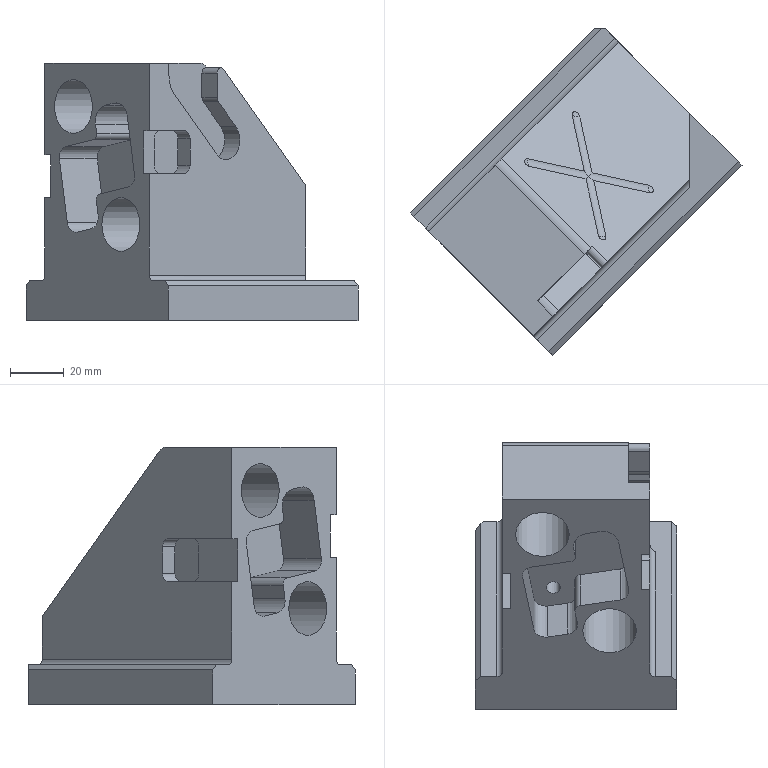Part | STEP file | gslz 2016.10.28-13_id346_x_t | 1 solid | 91 faces | box 123.744 x 121.622 x 96 mm | volume 385318 mm3 | plane 45 | cylinder 36 | sphere 4 | spline 4 | cone 2 | commonest cylinder face diameters 6 x16 4 x5 5.2 x3 20 x3 8 x2 9 x2